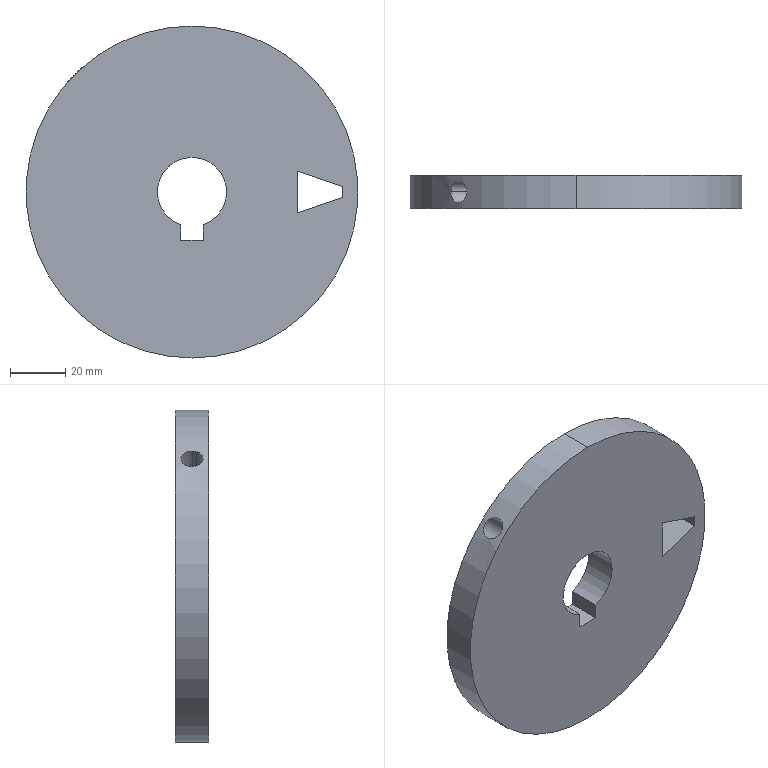Part | 1 solid | 18 faces | box 120 x 12 x 120 mm | volume 125702 mm3 | plane 10 | cylinder 8 | commonest cylinder face diameters 4.2 x2 8 x2 25 x2 120 x2
STEP:
#1=CARTESIAN_POINT('',(-10.198,6.,7.228));
#2=VERTEX_POINT('',#1);
#3=CARTESIAN_POINT('',(-7.228,6.,10.198));
#4=VERTEX_POINT('',#3);
#5=CARTESIAN_POINT('',(-10.198,6.,7.228));
#6=CARTESIAN_POINT('',(-10.198,5.726,7.228));
#7=CARTESIAN_POINT('',(-10.166,5.449,7.274));
#8=CARTESIAN_POINT('',(-10.072,5.07,7.403));
#9=CARTESIAN_POINT('',(-10.033,4.947,7.456));
#10=CARTESIAN_POINT('',(-9.94,4.718,7.579));
#11=CARTESIAN_POINT('',(-9.887,4.613,7.649));
#12=CARTESIAN_POINT('',(-9.767,4.419,7.802));
#13=CARTESIAN_POINT('',(-9.699,4.331,7.887));
#14=CARTESIAN_POINT('',(-9.553,4.178,8.063));
#15=CARTESIAN_POINT('',(-9.475,4.114,8.155));
#16=CARTESIAN_POINT('',(-9.306,4.008,8.346));
#17=CARTESIAN_POINT('',(-9.217,3.968,8.445));
#18=CARTESIAN_POINT('',(-9.033,3.914,8.641));
#19=CARTESIAN_POINT('',(-8.938,3.9,8.74));
#20=CARTESIAN_POINT('',(-8.742,3.9,8.936));
#21=CARTESIAN_POINT('',(-8.643,3.913,9.031));
#22=CARTESIAN_POINT('',(-8.447,3.967,9.215));
#23=CARTESIAN_POINT('',(-8.348,4.007,9.305));
#24=CARTESIAN_POINT('',(-8.157,4.112,9.473));
#25=CARTESIAN_POINT('',(-8.065,4.177,9.551));
#26=CARTESIAN_POINT('',(-7.888,4.329,9.698));
#27=CARTESIAN_POINT('',(-7.804,4.418,9.765));
#28=CARTESIAN_POINT('',(-7.574,4.707,9.946));
#29=CARTESIAN_POINT('',(-7.447,4.941,10.04));
#30=CARTESIAN_POINT('',(-7.318,5.32,10.134));
#31=CARTESIAN_POINT('',(-7.284,5.453,10.158));
#32=CARTESIAN_POINT('',(-7.24,5.724,10.19));
#33=CARTESIAN_POINT('',(-7.228,5.861,10.198));
#34=CARTESIAN_POINT('',(-7.228,6.,10.198));
#35=B_SPLINE_CURVE_WITH_KNOTS('',3,(#5,#6,#7,#8,#9,#10,#11,#12,#13,#14,#15,#16,#17,#18,#19,#20,#21,#22,#23,#24,#25,#26,#27,#28,#29,#30,#31,#32,#33,#34),.UNSPECIFIED.,.F.,.F.,(4,2,2,2,2,2,2,2,2,2,2,2,2,2,4),(0.006577,0.007399,0.00781,0.008221,0.008632,0.009043,0.009454,0.009865,0.01028,0.01069,0.0111,0.01151,0.01233,0.01274,0.01315),.UNSPECIFIED.);
#36=EDGE_CURVE('',#2,#4,#35,.T.);
#37=ORIENTED_EDGE('',*,*,#36,.F.);
#38=CARTESIAN_POINT('',(-22.698,6.,19.728));
#39=VERTEX_POINT('',#38);
#40=CARTESIAN_POINT('',(-22.698,6.,19.728));
#41=DIRECTION('',(-0.7071,0.,0.7071));
#42=VECTOR('',#41,1000.);
#43=LINE('',#40,#42);
#44=EDGE_CURVE('',#2,#39,#43,.T.);
#45=ORIENTED_EDGE('',*,*,#44,.T.);
#46=CARTESIAN_POINT('',(-19.728,6.,22.698));
#47=VERTEX_POINT('',#46);
#48=CARTESIAN_POINT('',(-21.213,6.,21.213));
#49=DIRECTION('',(-0.7071,0.,0.7071));
#50=DIRECTION('',(0.7071,0.,0.7071));
#51=AXIS2_PLACEMENT_3D('',#48,#49,#50);
#52=CIRCLE('',#51,2.1);
#53=EDGE_CURVE('',#39,#47,#52,.T.);
#54=ORIENTED_EDGE('',*,*,#53,.T.);
#55=CARTESIAN_POINT('',(-19.728,6.,22.698));
#56=DIRECTION('',(-0.7071,0.,0.7071));
#57=VECTOR('',#56,1000.);
#58=LINE('',#55,#57);
#59=EDGE_CURVE('',#4,#47,#58,.T.);
#60=ORIENTED_EDGE('',*,*,#59,.F.);
#61=EDGE_LOOP('',(#37,#45,#54,#60));
#62=FACE_OUTER_BOUND('',#61,.T.);
#63=CARTESIAN_POINT('',(-21.213,6.,21.213));
#64=DIRECTION('',(-0.7071,0.,0.7071));
#65=DIRECTION('',(0.7071,0.,0.7071));
#66=AXIS2_PLACEMENT_3D('',#63,#64,#65);
#67=CYLINDRICAL_SURFACE('',#66,2.1);
#68=ADVANCED_FACE('',(#62),#67,.F.);
#69=CARTESIAN_POINT('',(-24.042,6.,18.385));
#70=VERTEX_POINT('',#69);
#71=CARTESIAN_POINT('',(-18.385,6.,24.042));
#72=VERTEX_POINT('',#71);
#73=CARTESIAN_POINT('',(-21.213,6.,21.213));
#74=DIRECTION('',(-0.7071,0.,0.7071));
#75=DIRECTION('',(0.7071,0.,0.7071));
#76=AXIS2_PLACEMENT_3D('',#73,#74,#75);
#77=CIRCLE('',#76,4.);
#78=EDGE_CURVE('',#70,#72,#77,.T.);
#79=ORIENTED_EDGE('',*,*,#78,.F.);
#80=CARTESIAN_POINT('',(-45.16,6.,39.504));
#81=VERTEX_POINT('',#80);
#82=CARTESIAN_POINT('',(-24.042,6.,18.385));
#83=DIRECTION('',(-0.7071,0.,0.7071));
#84=VECTOR('',#83,1000.);
#85=LINE('',#82,#84);
#86=EDGE_CURVE('',#70,#81,#85,.T.);
#87=ORIENTED_EDGE('',*,*,#86,.T.);
#88=CARTESIAN_POINT('',(-39.504,6.,45.16));
#89=VERTEX_POINT('',#88);
#90=CARTESIAN_POINT('',(-39.504,6.,45.16));
#91=CARTESIAN_POINT('',(-39.504,5.736,45.16));
#92=CARTESIAN_POINT('',(-39.523,5.476,45.143));
#93=CARTESIAN_POINT('',(-39.6,4.964,45.076));
#94=CARTESIAN_POINT('',(-39.658,4.71,45.025));
#95=CARTESIAN_POINT('',(-39.809,4.226,44.892));
#96=CARTESIAN_POINT('',(-39.901,3.996,44.81));
#97=CARTESIAN_POINT('',(-40.117,3.561,44.616));
#98=CARTESIAN_POINT('',(-40.243,3.355,44.503));
#99=CARTESIAN_POINT('',(-40.516,2.987,44.255));
#100=CARTESIAN_POINT('',(-40.665,2.821,44.118));
#101=CARTESIAN_POINT('',(-40.985,2.529,43.821));
#102=CARTESIAN_POINT('',(-41.155,2.404,43.661));
#103=CARTESIAN_POINT('',(-41.504,2.205,43.33));
#104=CARTESIAN_POINT('',(-41.686,2.128,43.155));
#105=CARTESIAN_POINT('',(-42.056,2.025,42.794));
#106=CARTESIAN_POINT('',(-42.241,2.,42.612));
#107=CARTESIAN_POINT('',(-42.61,2.,42.243));
#108=CARTESIAN_POINT('',(-42.796,2.026,42.054));
#109=CARTESIAN_POINT('',(-43.154,2.128,41.687));
#110=CARTESIAN_POINT('',(-43.327,2.204,41.507));
#111=CARTESIAN_POINT('',(-43.661,2.404,41.156));
#112=CARTESIAN_POINT('',(-43.821,2.529,40.985));
#113=CARTESIAN_POINT('',(-44.116,2.819,40.667));
#114=CARTESIAN_POINT('',(-44.253,2.984,40.518));
#115=CARTESIAN_POINT('',(-44.505,3.358,40.241));
#116=CARTESIAN_POINT('',(-44.616,3.56,40.118));
#117=CARTESIAN_POINT('',(-44.809,3.993,39.902));
#118=CARTESIAN_POINT('',(-44.892,4.227,39.808));
#119=CARTESIAN_POINT('',(-45.026,4.712,39.657));
#120=CARTESIAN_POINT('',(-45.076,4.961,39.6));
#121=CARTESIAN_POINT('',(-45.143,5.474,39.523));
#122=CARTESIAN_POINT('',(-45.16,5.739,39.504));
#123=CARTESIAN_POINT('',(-45.16,6.,39.504));
#124=B_SPLINE_CURVE_WITH_KNOTS('',3,(#90,#91,#92,#93,#94,#95,#96,#97,#98,#99,#100,#101,#102,#103,#104,#105,#106,#107,#108,#109,#110,#111,#112,#113,#114,#115,#116,#117,#118,#119,#120,#121,#122,#123),.UNSPECIFIED.,.F.,.F.,(4,2,2,2,2,2,2,2,2,2,2,2,2,2,2,2,4),(0.,0.0007818,0.001564,0.002345,0.003127,0.003909,0.004691,0.005473,0.006255,0.007036,0.007818,0.0086,0.009382,0.01016,0.01095,0.01173,0.01251),.UNSPECIFIED.);
#125=EDGE_CURVE('',#89,#81,#124,.T.);
#126=ORIENTED_EDGE('',*,*,#125,.F.);
#127=CARTESIAN_POINT('',(-18.385,6.,24.042));
#128=DIRECTION('',(-0.7071,0.,0.7071));
#129=VECTOR('',#128,1000.);
#130=LINE('',#127,#129);
#131=EDGE_CURVE('',#72,#89,#130,.T.);
#132=ORIENTED_EDGE('',*,*,#131,.F.);
#133=EDGE_LOOP('',(#79,#87,#126,#132));
#134=FACE_OUTER_BOUND('',#133,.T.);
#135=CARTESIAN_POINT('',(-21.213,6.,21.213));
#136=DIRECTION('',(-0.7071,0.,0.7071));
#137=DIRECTION('',(0.7071,0.,0.7071));
#138=AXIS2_PLACEMENT_3D('',#135,#136,#137);
#139=CYLINDRICAL_SURFACE('',#138,4.);
#140=ADVANCED_FACE('',(#134),#139,.F.);
#141=CARTESIAN_POINT('',(0.,0.,12.5));
#142=VERTEX_POINT('',#141);
#143=CARTESIAN_POINT('',(4.,0.,-11.843));
#144=VERTEX_POINT('',#143);
#145=CARTESIAN_POINT('',(0.,0.,0.));
#146=DIRECTION('',(0.,1.,0.));
#147=DIRECTION('',(0.,0.,1.));
#148=AXIS2_PLACEMENT_3D('',#145,#146,#147);
#149=CIRCLE('',#148,12.5);
#150=EDGE_CURVE('',#142,#144,#149,.T.);
#151=ORIENTED_EDGE('',*,*,#150,.F.);
#152=CARTESIAN_POINT('',(0.,12.,12.5));
#153=VERTEX_POINT('',#152);
#154=CARTESIAN_POINT('',(0.,0.,12.5));
#155=DIRECTION('',(0.,1.,0.));
#156=VECTOR('',#155,1000.);
#157=LINE('',#154,#156);
#158=EDGE_CURVE('',#142,#153,#157,.T.);
#159=ORIENTED_EDGE('',*,*,#158,.T.);
#160=CARTESIAN_POINT('',(4.,12.,-11.843));
#161=VERTEX_POINT('',#160);
#162=CARTESIAN_POINT('',(0.,12.,0.));
#163=DIRECTION('',(0.,1.,0.));
#164=DIRECTION('',(0.,0.,1.));
#165=AXIS2_PLACEMENT_3D('',#162,#163,#164);
#166=CIRCLE('',#165,12.5);
#167=EDGE_CURVE('',#153,#161,#166,.T.);
#168=ORIENTED_EDGE('',*,*,#167,.T.);
#169=CARTESIAN_POINT('',(4.,0.,-11.843));
#170=DIRECTION('',(0.,1.,0.));
#171=VECTOR('',#170,1000.);
#172=LINE('',#169,#171);
#173=EDGE_CURVE('',#144,#161,#172,.T.);
#174=ORIENTED_EDGE('',*,*,#173,.F.);
#175=EDGE_LOOP('',(#151,#159,#168,#174));
#176=FACE_OUTER_BOUND('',#175,.T.);
#177=CARTESIAN_POINT('',(0.,0.,0.));
#178=DIRECTION('',(0.,1.,0.));
#179=DIRECTION('',(0.,0.,1.));
#180=AXIS2_PLACEMENT_3D('',#177,#178,#179);
#181=CYLINDRICAL_SURFACE('',#180,12.5);
#182=ADVANCED_FACE('',(#176),#181,.F.);
#183=CARTESIAN_POINT('',(0.,12.,60.));
#184=VERTEX_POINT('',#183);
#185=CARTESIAN_POINT('',(0.,12.,-60.));
#186=VERTEX_POINT('',#185);
#187=CARTESIAN_POINT('',(0.,12.,0.));
#188=DIRECTION('',(0.,1.,0.));
#189=DIRECTION('',(0.,0.,1.));
#190=AXIS2_PLACEMENT_3D('',#187,#188,#189);
#191=CIRCLE('',#190,60.);
#192=EDGE_CURVE('',#184,#186,#191,.T.);
#193=ORIENTED_EDGE('',*,*,#192,.F.);
#194=CARTESIAN_POINT('',(0.,0.,60.));
#195=VERTEX_POINT('',#194);
#196=CARTESIAN_POINT('',(0.,12.,60.));
#197=DIRECTION('',(0.,-1.,0.));
#198=VECTOR('',#197,1000.);
#199=LINE('',#196,#198);
#200=EDGE_CURVE('',#184,#195,#199,.T.);
#201=ORIENTED_EDGE('',*,*,#200,.T.);
#202=CARTESIAN_POINT('',(0.,0.,-60.));
#203=VERTEX_POINT('',#202);
#204=CARTESIAN_POINT('',(0.,0.,0.));
#205=DIRECTION('',(0.,1.,0.));
#206=DIRECTION('',(0.,0.,1.));
#207=AXIS2_PLACEMENT_3D('',#204,#205,#206);
#208=CIRCLE('',#207,60.);
#209=EDGE_CURVE('',#195,#203,#208,.T.);
#210=ORIENTED_EDGE('',*,*,#209,.T.);
#211=CARTESIAN_POINT('',(0.,12.,-60.));
#212=DIRECTION('',(0.,-1.,0.));
#213=VECTOR('',#212,1000.);
#214=LINE('',#211,#213);
#215=EDGE_CURVE('',#186,#203,#214,.T.);
#216=ORIENTED_EDGE('',*,*,#215,.F.);
#217=EDGE_LOOP('',(#193,#201,#210,#216));
#218=FACE_OUTER_BOUND('',#217,.T.);
#219=CARTESIAN_POINT('',(0.,12.,0.));
#220=DIRECTION('',(0.,-1.,0.));
#221=DIRECTION('',(0.,0.,-1.));
#222=AXIS2_PLACEMENT_3D('',#219,#220,#221);
#223=CYLINDRICAL_SURFACE('',#222,60.);
#224=ADVANCED_FACE('',(#218),#223,.T.);
#225=ORIENTED_EDGE('',*,*,#200,.F.);
#226=CARTESIAN_POINT('',(0.,12.,0.));
#227=DIRECTION('',(0.,1.,0.));
#228=DIRECTION('',(0.,0.,1.));
#229=AXIS2_PLACEMENT_3D('',#226,#227,#228);
#230=CIRCLE('',#229,60.);
#231=EDGE_CURVE('',#186,#184,#230,.T.);
#232=ORIENTED_EDGE('',*,*,#231,.F.);
#233=ORIENTED_EDGE('',*,*,#215,.T.);
#234=CARTESIAN_POINT('',(0.,0.,0.));
#235=DIRECTION('',(0.,1.,0.));
#236=DIRECTION('',(0.,0.,1.));
#237=AXIS2_PLACEMENT_3D('',#234,#235,#236);
#238=CIRCLE('',#237,60.);
#239=EDGE_CURVE('',#203,#195,#238,.T.);
#240=ORIENTED_EDGE('',*,*,#239,.T.);
#241=EDGE_LOOP('',(#225,#232,#233,#240));
#242=FACE_OUTER_BOUND('',#241,.T.);
#243=ORIENTED_EDGE('',*,*,#125,.T.);
#244=CARTESIAN_POINT('',(-45.16,6.,39.504));
#245=CARTESIAN_POINT('',(-45.16,6.261,39.504));
#246=CARTESIAN_POINT('',(-45.144,6.521,39.523));
#247=CARTESIAN_POINT('',(-45.076,7.036,39.6));
#248=CARTESIAN_POINT('',(-45.025,7.289,39.658));
#249=CARTESIAN_POINT('',(-44.893,7.77,39.807));
#250=CARTESIAN_POINT('',(-44.811,8.003,39.9));
#251=CARTESIAN_POINT('',(-44.616,8.441,40.118));
#252=CARTESIAN_POINT('',(-44.505,8.642,40.241));
#253=CARTESIAN_POINT('',(-44.256,9.011,40.514));
#254=CARTESIAN_POINT('',(-44.117,9.18,40.666));
#255=CARTESIAN_POINT('',(-43.821,9.471,40.985));
#256=CARTESIAN_POINT('',(-43.664,9.594,41.152));
#257=CARTESIAN_POINT('',(-43.331,9.794,41.503));
#258=CARTESIAN_POINT('',(-43.155,9.872,41.686));
#259=CARTESIAN_POINT('',(-42.798,9.974,42.053));
#260=CARTESIAN_POINT('',(-42.615,10.,42.237));
#261=CARTESIAN_POINT('',(-42.242,10.,42.611));
#262=CARTESIAN_POINT('',(-42.056,9.974,42.794));
#263=CARTESIAN_POINT('',(-41.69,9.873,43.151));
#264=CARTESIAN_POINT('',(-41.507,9.797,43.327));
#265=CARTESIAN_POINT('',(-41.156,9.596,43.661));
#266=CARTESIAN_POINT('',(-40.988,9.473,43.818));
#267=CARTESIAN_POINT('',(-40.669,9.184,44.114));
#268=CARTESIAN_POINT('',(-40.517,9.015,44.253));
#269=CARTESIAN_POINT('',(-40.244,8.646,44.502));
#270=CARTESIAN_POINT('',(-40.121,8.445,44.613));
#271=CARTESIAN_POINT('',(-39.902,8.008,44.809));
#272=CARTESIAN_POINT('',(-39.809,7.775,44.892));
#273=CARTESIAN_POINT('',(-39.659,7.294,45.024));
#274=CARTESIAN_POINT('',(-39.601,7.043,45.075));
#275=CARTESIAN_POINT('',(-39.523,6.526,45.143));
#276=CARTESIAN_POINT('',(-39.504,6.264,45.16));
#277=CARTESIAN_POINT('',(-39.504,6.,45.16));
#278=B_SPLINE_CURVE_WITH_KNOTS('',3,(#244,#245,#246,#247,#248,#249,#250,#251,#252,#253,#254,#255,#256,#257,#258,#259,#260,#261,#262,#263,#264,#265,#266,#267,#268,#269,#270,#271,#272,#273,#274,#275,#276,#277),.UNSPECIFIED.,.F.,.F.,(4,2,2,2,2,2,2,2,2,2,2,2,2,2,2,2,4),(0.01251,0.01329,0.01407,0.01485,0.01564,0.01642,0.0172,0.01798,0.01876,0.01954,0.02033,0.02111,0.02189,0.02267,0.02345,0.02423,0.02502),.UNSPECIFIED.);
#279=EDGE_CURVE('',#81,#89,#278,.T.);
#280=ORIENTED_EDGE('',*,*,#279,.T.);
#281=EDGE_LOOP('',(#243,#280));
#282=FACE_BOUND('',#281,.T.);
#283=CARTESIAN_POINT('',(0.,12.,0.));
#284=DIRECTION('',(0.,-1.,0.));
#285=DIRECTION('',(0.,0.,-1.));
#286=AXIS2_PLACEMENT_3D('',#283,#284,#285);
#287=CYLINDRICAL_SURFACE('',#286,60.);
#288=ADVANCED_FACE('',(#242,#282),#287,.T.);
#289=CARTESIAN_POINT('',(38.,12.,-7.5));
#290=VERTEX_POINT('',#289);
#291=CARTESIAN_POINT('',(38.,12.,7.5));
#292=VERTEX_POINT('',#291);
#293=CARTESIAN_POINT('',(38.,12.,7.5));
#294=DIRECTION('',(0.,0.,1.));
#295=VECTOR('',#294,1000.);
#296=LINE('',#293,#295);
#297=EDGE_CURVE('',#290,#292,#296,.T.);
#298=ORIENTED_EDGE('',*,*,#297,.F.);
#299=CARTESIAN_POINT('',(54.438,12.,-2.));
#300=VERTEX_POINT('',#299);
#301=CARTESIAN_POINT('',(38.,12.,-7.5));
#302=DIRECTION('',(-0.9483,0.,-0.3173));
#303=VECTOR('',#302,1000.);
#304=LINE('',#301,#303);
#305=EDGE_CURVE('',#300,#290,#304,.T.);
#306=ORIENTED_EDGE('',*,*,#305,.F.);
#307=CARTESIAN_POINT('',(54.438,12.,2.));
#308=VERTEX_POINT('',#307);
#309=CARTESIAN_POINT('',(54.438,12.,-2.));
#310=DIRECTION('',(0.,0.,-1.));
#311=VECTOR('',#310,1000.);
#312=LINE('',#309,#311);
#313=EDGE_CURVE('',#308,#300,#312,.T.);
#314=ORIENTED_EDGE('',*,*,#313,.F.);
#315=CARTESIAN_POINT('',(54.438,12.,2.));
#316=DIRECTION('',(0.9483,0.,-0.3173));
#317=VECTOR('',#316,1000.);
#318=LINE('',#315,#317);
#319=EDGE_CURVE('',#292,#308,#318,.T.);
#320=ORIENTED_EDGE('',*,*,#319,.F.);
#321=EDGE_LOOP('',(#298,#306,#314,#320));
#322=FACE_BOUND('',#321,.T.);
#323=CARTESIAN_POINT('',(-4.,12.,-11.843));
#324=VERTEX_POINT('',#323);
#325=CARTESIAN_POINT('',(0.,12.,0.));
#326=DIRECTION('',(0.,1.,0.));
#327=DIRECTION('',(0.,0.,1.));
#328=AXIS2_PLACEMENT_3D('',#325,#326,#327);
#329=CIRCLE('',#328,12.5);
#330=EDGE_CURVE('',#324,#153,#329,.T.);
#331=ORIENTED_EDGE('',*,*,#330,.F.);
#332=CARTESIAN_POINT('',(-4.,12.,-17.5));
#333=VERTEX_POINT('',#332);
#334=CARTESIAN_POINT('',(-4.,12.,-11.843));
#335=DIRECTION('',(0.,0.,1.));
#336=VECTOR('',#335,1000.);
#337=LINE('',#334,#336);
#338=EDGE_CURVE('',#333,#324,#337,.T.);
#339=ORIENTED_EDGE('',*,*,#338,.F.);
#340=CARTESIAN_POINT('',(4.,12.,-17.5));
#341=VERTEX_POINT('',#340);
#342=CARTESIAN_POINT('',(-4.,12.,-17.5));
#343=DIRECTION('',(-1.,0.,0.));
#344=VECTOR('',#343,1000.);
#345=LINE('',#342,#344);
#346=EDGE_CURVE('',#341,#333,#345,.T.);
#347=ORIENTED_EDGE('',*,*,#346,.F.);
#348=CARTESIAN_POINT('',(4.,12.,-17.5));
#349=DIRECTION('',(0.,0.,-1.));
#350=VECTOR('',#349,1000.);
#351=LINE('',#348,#350);
#352=EDGE_CURVE('',#161,#341,#351,.T.);
#353=ORIENTED_EDGE('',*,*,#352,.F.);
#354=ORIENTED_EDGE('',*,*,#167,.F.);
#355=EDGE_LOOP('',(#331,#339,#347,#353,#354));
#356=FACE_BOUND('',#355,.T.);
#357=ORIENTED_EDGE('',*,*,#231,.T.);
#358=ORIENTED_EDGE('',*,*,#192,.T.);
#359=EDGE_LOOP('',(#357,#358));
#360=FACE_OUTER_BOUND('',#359,.T.);
#361=CARTESIAN_POINT('',(0.,12.,0.));
#362=DIRECTION('',(0.,1.,0.));
#363=DIRECTION('',(0.,0.,1.));
#364=AXIS2_PLACEMENT_3D('',#361,#362,#363);
#365=PLANE('',#364);
#366=ADVANCED_FACE('',(#322,#356,#360),#365,.T.);
#367=CARTESIAN_POINT('',(54.438,0.,-2.));
#368=VERTEX_POINT('',#367);
#369=CARTESIAN_POINT('',(38.,0.,-7.5));
#370=VERTEX_POINT('',#369);
#371=CARTESIAN_POINT('',(38.,0.,-7.5));
#372=DIRECTION('',(-0.9483,0.,-0.3173));
#373=VECTOR('',#372,1000.);
#374=LINE('',#371,#373);
#375=EDGE_CURVE('',#368,#370,#374,.T.);
#376=ORIENTED_EDGE('',*,*,#375,.T.);
#377=CARTESIAN_POINT('',(38.,0.,7.5));
#378=VERTEX_POINT('',#377);
#379=CARTESIAN_POINT('',(38.,0.,7.5));
#380=DIRECTION('',(0.,0.,1.));
#381=VECTOR('',#380,1000.);
#382=LINE('',#379,#381);
#383=EDGE_CURVE('',#370,#378,#382,.T.);
#384=ORIENTED_EDGE('',*,*,#383,.T.);
#385=CARTESIAN_POINT('',(54.438,0.,2.));
#386=VERTEX_POINT('',#385);
#387=CARTESIAN_POINT('',(54.438,0.,2.));
#388=DIRECTION('',(0.9483,0.,-0.3173));
#389=VECTOR('',#388,1000.);
#390=LINE('',#387,#389);
#391=EDGE_CURVE('',#378,#386,#390,.T.);
#392=ORIENTED_EDGE('',*,*,#391,.T.);
#393=CARTESIAN_POINT('',(54.438,0.,-2.));
#394=DIRECTION('',(0.,0.,-1.));
#395=VECTOR('',#394,1000.);
#396=LINE('',#393,#395);
#397=EDGE_CURVE('',#386,#368,#396,.T.);
#398=ORIENTED_EDGE('',*,*,#397,.T.);
#399=EDGE_LOOP('',(#376,#384,#392,#398));
#400=FACE_BOUND('',#399,.T.);
#401=CARTESIAN_POINT('',(-4.,0.,-17.5));
#402=VERTEX_POINT('',#401);
#403=CARTESIAN_POINT('',(-4.,0.,-11.843));
#404=VERTEX_POINT('',#403);
#405=CARTESIAN_POINT('',(-4.,0.,-11.843));
#406=DIRECTION('',(0.,0.,1.));
#407=VECTOR('',#406,1000.);
#408=LINE('',#405,#407);
#409=EDGE_CURVE('',#402,#404,#408,.T.);
#410=ORIENTED_EDGE('',*,*,#409,.T.);
#411=CARTESIAN_POINT('',(0.,0.,0.));
#412=DIRECTION('',(0.,1.,0.));
#413=DIRECTION('',(0.,0.,1.));
#414=AXIS2_PLACEMENT_3D('',#411,#412,#413);
#415=CIRCLE('',#414,12.5);
#416=EDGE_CURVE('',#404,#142,#415,.T.);
#417=ORIENTED_EDGE('',*,*,#416,.T.);
#418=ORIENTED_EDGE('',*,*,#150,.T.);
#419=CARTESIAN_POINT('',(4.,0.,-17.5));
#420=VERTEX_POINT('',#419);
#421=CARTESIAN_POINT('',(4.,0.,-17.5));
#422=DIRECTION('',(0.,0.,-1.));
#423=VECTOR('',#422,1000.);
#424=LINE('',#421,#423);
#425=EDGE_CURVE('',#144,#420,#424,.T.);
#426=ORIENTED_EDGE('',*,*,#425,.T.);
#427=CARTESIAN_POINT('',(-4.,0.,-17.5));
#428=DIRECTION('',(-1.,0.,0.));
#429=VECTOR('',#428,1000.);
#430=LINE('',#427,#429);
#431=EDGE_CURVE('',#420,#402,#430,.T.);
#432=ORIENTED_EDGE('',*,*,#431,.T.);
#433=EDGE_LOOP('',(#410,#417,#418,#426,#432));
#434=FACE_BOUND('',#433,.T.);
#435=ORIENTED_EDGE('',*,*,#239,.F.);
#436=ORIENTED_EDGE('',*,*,#209,.F.);
#437=EDGE_LOOP('',(#435,#436));
#438=FACE_OUTER_BOUND('',#437,.T.);
#439=CARTESIAN_POINT('',(0.,0.,0.));
#440=DIRECTION('',(0.,1.,0.));
#441=DIRECTION('',(0.,0.,1.));
#442=AXIS2_PLACEMENT_3D('',#439,#440,#441);
#443=PLANE('',#442);
#444=ADVANCED_FACE('',(#400,#434,#438),#443,.F.);
#445=ORIENTED_EDGE('',*,*,#158,.F.);
#446=ORIENTED_EDGE('',*,*,#416,.F.);
#447=CARTESIAN_POINT('',(-4.,0.,-11.843));
#448=DIRECTION('',(0.,1.,0.));
#449=VECTOR('',#448,1000.);
#450=LINE('',#447,#449);
#451=EDGE_CURVE('',#404,#324,#450,.T.);
#452=ORIENTED_EDGE('',*,*,#451,.T.);
#453=ORIENTED_EDGE('',*,*,#330,.T.);
#454=EDGE_LOOP('',(#445,#446,#452,#453));
#455=FACE_OUTER_BOUND('',#454,.T.);
#456=CARTESIAN_POINT('',(-7.228,6.,10.198));
#457=CARTESIAN_POINT('',(-7.228,6.139,10.198));
#458=CARTESIAN_POINT('',(-7.24,6.276,10.19));
#459=CARTESIAN_POINT('',(-7.284,6.544,10.159));
#460=CARTESIAN_POINT('',(-7.317,6.678,10.135));
#461=CARTESIAN_POINT('',(-7.403,6.932,10.072));
#462=CARTESIAN_POINT('',(-7.456,7.053,10.033));
#463=CARTESIAN_POINT('',(-7.579,7.281,9.941));
#464=CARTESIAN_POINT('',(-7.65,7.389,9.886));
#465=CARTESIAN_POINT('',(-7.88,7.679,9.706));
#466=CARTESIAN_POINT('',(-8.061,7.835,9.557));
#467=CARTESIAN_POINT('',(-8.442,8.045,9.222));
#468=CARTESIAN_POINT('',(-8.644,8.1,9.033));
#469=CARTESIAN_POINT('',(-8.935,8.1,8.742));
#470=CARTESIAN_POINT('',(-9.032,8.086,8.642));
#471=CARTESIAN_POINT('',(-9.217,8.033,8.445));
#472=CARTESIAN_POINT('',(-9.305,7.993,8.348));
#473=CARTESIAN_POINT('',(-9.473,7.887,8.156));
#474=CARTESIAN_POINT('',(-9.553,7.822,8.063));
#475=CARTESIAN_POINT('',(-9.698,7.67,7.887));
#476=CARTESIAN_POINT('',(-9.765,7.583,7.804));
#477=CARTESIAN_POINT('',(-9.887,7.387,7.649));
#478=CARTESIAN_POINT('',(-9.94,7.281,7.579));
#479=CARTESIAN_POINT('',(-10.033,7.054,7.457));
#480=CARTESIAN_POINT('',(-10.072,6.931,7.403));
#481=CARTESIAN_POINT('',(-10.135,6.677,7.317));
#482=CARTESIAN_POINT('',(-10.158,6.546,7.284));
#483=CARTESIAN_POINT('',(-10.19,6.277,7.24));
#484=CARTESIAN_POINT('',(-10.198,6.137,7.228));
#485=CARTESIAN_POINT('',(-10.198,6.,7.228));
#486=B_SPLINE_CURVE_WITH_KNOTS('',3,(#456,#457,#458,#459,#460,#461,#462,#463,#464,#465,#466,#467,#468,#469,#470,#471,#472,#473,#474,#475,#476,#477,#478,#479,#480,#481,#482,#483,#484,#485),.UNSPECIFIED.,.F.,.F.,(4,2,2,2,2,2,2,2,2,2,2,2,2,2,4),(0.,0.0004111,0.0008222,0.001233,0.001644,0.002466,0.003289,0.0037,0.004111,0.004522,0.004933,0.005344,0.005755,0.006166,0.006577),.UNSPECIFIED.);
#487=EDGE_CURVE('',#4,#2,#486,.T.);
#488=ORIENTED_EDGE('',*,*,#487,.T.);
#489=ORIENTED_EDGE('',*,*,#36,.T.);
#490=EDGE_LOOP('',(#488,#489));
#491=FACE_BOUND('',#490,.T.);
#492=CARTESIAN_POINT('',(0.,0.,0.));
#493=DIRECTION('',(0.,1.,0.));
#494=DIRECTION('',(0.,0.,1.));
#495=AXIS2_PLACEMENT_3D('',#492,#493,#494);
#496=CYLINDRICAL_SURFACE('',#495,12.5);
#497=ADVANCED_FACE('',(#455,#491),#496,.F.);
#498=ORIENTED_EDGE('',*,*,#338,.T.);
#499=ORIENTED_EDGE('',*,*,#451,.F.);
#500=ORIENTED_EDGE('',*,*,#409,.F.);
#501=CARTESIAN_POINT('',(-4.,0.,-17.5));
#502=DIRECTION('',(0.,1.,0.));
#503=VECTOR('',#502,1000.);
#504=LINE('',#501,#503);
#505=EDGE_CURVE('',#402,#333,#504,.T.);
#506=ORIENTED_EDGE('',*,*,#505,.T.);
#507=EDGE_LOOP('',(#498,#499,#500,#506));
#508=FACE_OUTER_BOUND('',#507,.T.);
#509=CARTESIAN_POINT('',(-4.,0.,-11.843));
#510=DIRECTION('',(-1.,0.,0.));
#511=DIRECTION('',(0.,0.,1.));
#512=AXIS2_PLACEMENT_3D('',#509,#510,#511);
#513=PLANE('',#512);
#514=ADVANCED_FACE('',(#508),#513,.F.);
#515=ORIENTED_EDGE('',*,*,#346,.T.);
#516=ORIENTED_EDGE('',*,*,#505,.F.);
#517=ORIENTED_EDGE('',*,*,#431,.F.);
#518=CARTESIAN_POINT('',(4.,0.,-17.5));
#519=DIRECTION('',(0.,1.,0.));
#520=VECTOR('',#519,1000.);
#521=LINE('',#518,#520);
#522=EDGE_CURVE('',#420,#341,#521,.T.);
#523=ORIENTED_EDGE('',*,*,#522,.T.);
#524=EDGE_LOOP('',(#515,#516,#517,#523));
#525=FACE_OUTER_BOUND('',#524,.T.);
#526=CARTESIAN_POINT('',(-4.,0.,-17.5));
#527=DIRECTION('',(0.,0.,-1.));
#528=DIRECTION('',(-1.,0.,0.));
#529=AXIS2_PLACEMENT_3D('',#526,#527,#528);
#530=PLANE('',#529);
#531=ADVANCED_FACE('',(#525),#530,.F.);
#532=ORIENTED_EDGE('',*,*,#352,.T.);
#533=ORIENTED_EDGE('',*,*,#522,.F.);
#534=ORIENTED_EDGE('',*,*,#425,.F.);
#535=ORIENTED_EDGE('',*,*,#173,.T.);
#536=EDGE_LOOP('',(#532,#533,#534,#535));
#537=FACE_OUTER_BOUND('',#536,.T.);
#538=CARTESIAN_POINT('',(4.,0.,-17.5));
#539=DIRECTION('',(1.,0.,0.));
#540=DIRECTION('',(0.,0.,-1.));
#541=AXIS2_PLACEMENT_3D('',#538,#539,#540);
#542=PLANE('',#541);
#543=ADVANCED_FACE('',(#537),#542,.F.);
#544=ORIENTED_EDGE('',*,*,#297,.T.);
#545=CARTESIAN_POINT('',(38.,0.,7.5));
#546=DIRECTION('',(0.,1.,0.));
#547=VECTOR('',#546,1000.);
#548=LINE('',#545,#547);
#549=EDGE_CURVE('',#378,#292,#548,.T.);
#550=ORIENTED_EDGE('',*,*,#549,.F.);
#551=ORIENTED_EDGE('',*,*,#383,.F.);
#552=CARTESIAN_POINT('',(38.,0.,-7.5));
#553=DIRECTION('',(0.,1.,0.));
#554=VECTOR('',#553,1000.);
#555=LINE('',#552,#554);
#556=EDGE_CURVE('',#370,#290,#555,.T.);
#557=ORIENTED_EDGE('',*,*,#556,.T.);
#558=EDGE_LOOP('',(#544,#550,#551,#557));
#559=FACE_OUTER_BOUND('',#558,.T.);
#560=CARTESIAN_POINT('',(38.,0.,7.5));
#561=DIRECTION('',(-1.,0.,0.));
#562=DIRECTION('',(0.,0.,1.));
#563=AXIS2_PLACEMENT_3D('',#560,#561,#562);
#564=PLANE('',#563);
#565=ADVANCED_FACE('',(#559),#564,.F.);
#566=ORIENTED_EDGE('',*,*,#305,.T.);
#567=ORIENTED_EDGE('',*,*,#556,.F.);
#568=ORIENTED_EDGE('',*,*,#375,.F.);
#569=CARTESIAN_POINT('',(54.438,0.,-2.));
#570=DIRECTION('',(0.,1.,0.));
#571=VECTOR('',#570,1000.);
#572=LINE('',#569,#571);
#573=EDGE_CURVE('',#368,#300,#572,.T.);
#574=ORIENTED_EDGE('',*,*,#573,.T.);
#575=EDGE_LOOP('',(#566,#567,#568,#574));
#576=FACE_OUTER_BOUND('',#575,.T.);
#577=CARTESIAN_POINT('',(38.,0.,-7.5));
#578=DIRECTION('',(0.3173,0.,-0.9483));
#579=DIRECTION('',(-0.9483,0.,-0.3173));
#580=AXIS2_PLACEMENT_3D('',#577,#578,#579);
#581=PLANE('',#580);
#582=ADVANCED_FACE('',(#576),#581,.F.);
#583=ORIENTED_EDGE('',*,*,#313,.T.);
#584=ORIENTED_EDGE('',*,*,#573,.F.);
#585=ORIENTED_EDGE('',*,*,#397,.F.);
#586=CARTESIAN_POINT('',(54.438,0.,2.));
#587=DIRECTION('',(0.,1.,0.));
#588=VECTOR('',#587,1000.);
#589=LINE('',#586,#588);
#590=EDGE_CURVE('',#386,#308,#589,.T.);
#591=ORIENTED_EDGE('',*,*,#590,.T.);
#592=EDGE_LOOP('',(#583,#584,#585,#591));
#593=FACE_OUTER_BOUND('',#592,.T.);
#594=CARTESIAN_POINT('',(54.438,0.,-2.));
#595=DIRECTION('',(1.,0.,0.));
#596=DIRECTION('',(0.,0.,-1.));
#597=AXIS2_PLACEMENT_3D('',#594,#595,#596);
#598=PLANE('',#597);
#599=ADVANCED_FACE('',(#593),#598,.F.);
#600=ORIENTED_EDGE('',*,*,#319,.T.);
#601=ORIENTED_EDGE('',*,*,#590,.F.);
#602=ORIENTED_EDGE('',*,*,#391,.F.);
#603=ORIENTED_EDGE('',*,*,#549,.T.);
#604=EDGE_LOOP('',(#600,#601,#602,#603));
#605=FACE_OUTER_BOUND('',#604,.T.);
#606=CARTESIAN_POINT('',(54.438,0.,2.));
#607=DIRECTION('',(0.3173,0.,0.9483));
#608=DIRECTION('',(0.9483,0.,-0.3173));
#609=AXIS2_PLACEMENT_3D('',#606,#607,#608);
#610=PLANE('',#609);
#611=ADVANCED_FACE('',(#605),#610,.F.);
#612=ORIENTED_EDGE('',*,*,#86,.F.);
#613=CARTESIAN_POINT('',(-21.213,6.,21.213));
#614=DIRECTION('',(-0.7071,0.,0.7071));
#615=DIRECTION('',(0.7071,0.,0.7071));
#616=AXIS2_PLACEMENT_3D('',#613,#614,#615);
#617=CIRCLE('',#616,4.);
#618=EDGE_CURVE('',#72,#70,#617,.T.);
#619=ORIENTED_EDGE('',*,*,#618,.F.);
#620=ORIENTED_EDGE('',*,*,#131,.T.);
#621=ORIENTED_EDGE('',*,*,#279,.F.);
#622=EDGE_LOOP('',(#612,#619,#620,#621));
#623=FACE_OUTER_BOUND('',#622,.T.);
#624=CARTESIAN_POINT('',(-21.213,6.,21.213));
#625=DIRECTION('',(-0.7071,0.,0.7071));
#626=DIRECTION('',(0.7071,0.,0.7071));
#627=AXIS2_PLACEMENT_3D('',#624,#625,#626);
#628=CYLINDRICAL_SURFACE('',#627,4.);
#629=ADVANCED_FACE('',(#623),#628,.F.);
#630=CARTESIAN_POINT('',(-21.213,6.,21.213));
#631=DIRECTION('',(-0.7071,0.,0.7071));
#632=DIRECTION('',(0.7071,0.,0.7071));
#633=AXIS2_PLACEMENT_3D('',#630,#631,#632);
#634=CIRCLE('',#633,2.1);
#635=EDGE_CURVE('',#47,#39,#634,.T.);
#636=ORIENTED_EDGE('',*,*,#635,.F.);
#637=ORIENTED_EDGE('',*,*,#53,.F.);
#638=EDGE_LOOP('',(#636,#637));
#639=FACE_BOUND('',#638,.T.);
#640=ORIENTED_EDGE('',*,*,#618,.T.);
#641=ORIENTED_EDGE('',*,*,#78,.T.);
#642=EDGE_LOOP('',(#640,#641));
#643=FACE_OUTER_BOUND('',#642,.T.);
#644=CARTESIAN_POINT('',(-21.213,6.,21.213));
#645=DIRECTION('',(-0.7071,0.,0.7071));
#646=DIRECTION('',(0.7071,0.,0.7071));
#647=AXIS2_PLACEMENT_3D('',#644,#645,#646);
#648=PLANE('',#647);
#649=ADVANCED_FACE('',(#639,#643),#648,.T.);
#650=ORIENTED_EDGE('',*,*,#44,.F.);
#651=ORIENTED_EDGE('',*,*,#487,.F.);
#652=ORIENTED_EDGE('',*,*,#59,.T.);
#653=ORIENTED_EDGE('',*,*,#635,.T.);
#654=EDGE_LOOP('',(#650,#651,#652,#653));
#655=FACE_OUTER_BOUND('',#654,.T.);
#656=CARTESIAN_POINT('',(-21.213,6.,21.213));
#657=DIRECTION('',(-0.7071,0.,0.7071));
#658=DIRECTION('',(0.7071,0.,0.7071));
#659=AXIS2_PLACEMENT_3D('',#656,#657,#658);
#660=CYLINDRICAL_SURFACE('',#659,2.1);
#661=ADVANCED_FACE('',(#655),#660,.F.);
#662=CLOSED_SHELL('',(#68,#140,#182,#224,#288,#366,#444,#497,#514,#531,#543,#565,#582,#599,#611,#629,#649,#661));
#663=MANIFOLD_SOLID_BREP('',#662);
#664=CARTESIAN_POINT('',(0.,0.,0.));
#665=DIRECTION('',(0.,0.,1.));
#666=DIRECTION('',(1.,0.,0.));
#667=AXIS2_PLACEMENT_3D('',#664,#665,#666);
#668=(LENGTH_UNIT()NAMED_UNIT(*)SI_UNIT(.MILLI.,.METRE.));
#669=UNCERTAINTY_MEASURE_WITH_UNIT(LENGTH_MEASURE(0.00001),#668,'','');
#670=(NAMED_UNIT(*)PLANE_ANGLE_UNIT()SI_UNIT($,.RADIAN.));
#671=(NAMED_UNIT(*)SI_UNIT($,.STERADIAN.)SOLID_ANGLE_UNIT());
#672=(GEOMETRIC_REPRESENTATION_CONTEXT(3)GLOBAL_UNCERTAINTY_ASSIGNED_CONTEXT((#669))GLOBAL_UNIT_ASSIGNED_CONTEXT((#668,#670,#671))REPRESENTATION_CONTEXT('',''));
#673=ADVANCED_BREP_SHAPE_REPRESENTATION('',(#663,#667),#672);